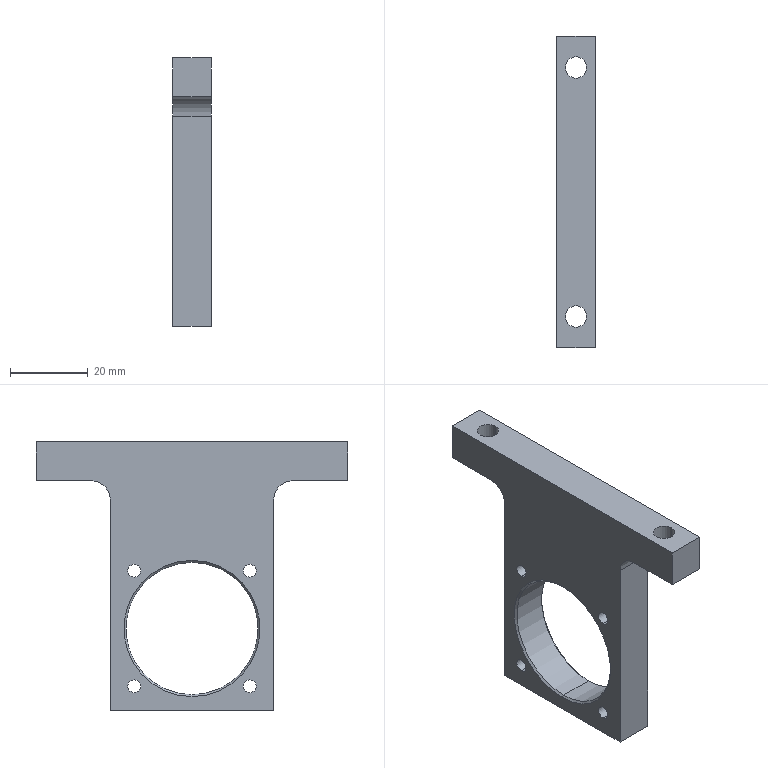Part | SolidWorks | features HoleWzd 2, Chamfer 1, Extrusion 1, Fillet 1, ICE 1 | 1 solid | 30 faces | box 10 x 80 x 69 mm | volume 22964 mm3 | cylinder 16 | plane 10 | cone 4 | commonest cylinder face diameters 3.3 x8 5.5 x4 10 x2 34 x2
STEP:
#1=CARTESIAN_POINT('',(9.5,0.,-31.));
#2=VERTEX_POINT('',#1);
#3=CARTESIAN_POINT('',(9.5,0.,-65.));
#4=VERTEX_POINT('',#3);
#5=CARTESIAN_POINT('',(9.5,0.,-48.));
#6=DIRECTION('',(1.,0.,0.));
#7=DIRECTION('',(0.,0.,1.));
#8=AXIS2_PLACEMENT_3D('',#5,#6,#7);
#9=CIRCLE('',#8,17.);
#10=EDGE_CURVE('',#2,#4,#9,.T.);
#11=ORIENTED_EDGE('',*,*,#10,.F.);
#12=CARTESIAN_POINT('',(10.,0.,-30.5));
#13=VERTEX_POINT('',#12);
#14=CARTESIAN_POINT('',(9.5,0.,-31.));
#15=DIRECTION('',(0.7071,0.,0.7071));
#16=VECTOR('',#15,1000.);
#17=LINE('',#14,#16);
#18=EDGE_CURVE('',#2,#13,#17,.T.);
#19=ORIENTED_EDGE('',*,*,#18,.T.);
#20=CARTESIAN_POINT('',(10.,0.,-65.5));
#21=VERTEX_POINT('',#20);
#22=CARTESIAN_POINT('',(10.,0.,-48.));
#23=DIRECTION('',(-1.,0.,0.));
#24=DIRECTION('',(0.,0.,1.));
#25=AXIS2_PLACEMENT_3D('',#22,#23,#24);
#26=CIRCLE('',#25,17.5);
#27=EDGE_CURVE('',#21,#13,#26,.T.);
#28=ORIENTED_EDGE('',*,*,#27,.F.);
#29=CARTESIAN_POINT('',(9.5,0.,-65.));
#30=DIRECTION('',(0.7071,0.,-0.7071));
#31=VECTOR('',#30,1000.);
#32=LINE('',#29,#31);
#33=EDGE_CURVE('',#4,#21,#32,.T.);
#34=ORIENTED_EDGE('',*,*,#33,.F.);
#35=EDGE_LOOP('',(#11,#19,#28,#34));
#36=FACE_OUTER_BOUND('',#35,.T.);
#37=CARTESIAN_POINT('',(9.5,0.,-48.));
#38=DIRECTION('',(1.,0.,0.));
#39=DIRECTION('',(0.,0.,-1.));
#40=AXIS2_PLACEMENT_3D('',#37,#38,#39);
#41=CONICAL_SURFACE('',#40,17.,0.7854);
#42=ADVANCED_FACE('',(#36),#41,.F.);
#43=CARTESIAN_POINT('',(0.5,0.,-65.));
#44=VERTEX_POINT('',#43);
#45=CARTESIAN_POINT('',(0.5,0.,-31.));
#46=VERTEX_POINT('',#45);
#47=CARTESIAN_POINT('',(0.5,0.,-48.));
#48=DIRECTION('',(-1.,0.,0.));
#49=DIRECTION('',(0.,0.,1.));
#50=AXIS2_PLACEMENT_3D('',#47,#48,#49);
#51=CIRCLE('',#50,17.);
#52=EDGE_CURVE('',#44,#46,#51,.T.);
#53=ORIENTED_EDGE('',*,*,#52,.F.);
#54=CARTESIAN_POINT('',(0.,0.,-65.5));
#55=VERTEX_POINT('',#54);
#56=CARTESIAN_POINT('',(0.,0.,-65.5));
#57=DIRECTION('',(-0.7071,0.,-0.7071));
#58=VECTOR('',#57,1000.);
#59=LINE('',#56,#58);
#60=EDGE_CURVE('',#44,#55,#59,.T.);
#61=ORIENTED_EDGE('',*,*,#60,.T.);
#62=CARTESIAN_POINT('',(0.,0.,-30.5));
#63=VERTEX_POINT('',#62);
#64=CARTESIAN_POINT('',(0.,0.,-48.));
#65=DIRECTION('',(1.,0.,0.));
#66=DIRECTION('',(0.,0.,1.));
#67=AXIS2_PLACEMENT_3D('',#64,#65,#66);
#68=CIRCLE('',#67,17.5);
#69=EDGE_CURVE('',#63,#55,#68,.T.);
#70=ORIENTED_EDGE('',*,*,#69,.F.);
#71=CARTESIAN_POINT('',(0.,0.,-30.5));
#72=DIRECTION('',(-0.7071,0.,0.7071));
#73=VECTOR('',#72,1000.);
#74=LINE('',#71,#73);
#75=EDGE_CURVE('',#46,#63,#74,.T.);
#76=ORIENTED_EDGE('',*,*,#75,.F.);
#77=EDGE_LOOP('',(#53,#61,#70,#76));
#78=FACE_OUTER_BOUND('',#77,.T.);
#79=CARTESIAN_POINT('',(0.,0.,-48.));
#80=DIRECTION('',(-1.,0.,0.));
#81=DIRECTION('',(0.,0.,1.));
#82=AXIS2_PLACEMENT_3D('',#79,#80,#81);
#83=CONICAL_SURFACE('',#82,17.5,0.7854);
#84=ADVANCED_FACE('',(#78),#83,.F.);
#85=CARTESIAN_POINT('',(0.,14.849,-31.501));
#86=VERTEX_POINT('',#85);
#87=CARTESIAN_POINT('',(0.,14.849,-34.801));
#88=VERTEX_POINT('',#87);
#89=CARTESIAN_POINT('',(0.,14.849,-33.151));
#90=DIRECTION('',(1.,0.,0.));
#91=DIRECTION('',(0.,0.,-1.));
#92=AXIS2_PLACEMENT_3D('',#89,#90,#91);
#93=CIRCLE('',#92,1.65);
#94=EDGE_CURVE('',#86,#88,#93,.T.);
#95=ORIENTED_EDGE('',*,*,#94,.F.);
#96=CARTESIAN_POINT('',(10.,14.849,-31.501));
#97=VERTEX_POINT('',#96);
#98=CARTESIAN_POINT('',(10.,14.849,-31.501));
#99=DIRECTION('',(1.,0.,0.));
#100=VECTOR('',#99,1000.);
#101=LINE('',#98,#100);
#102=EDGE_CURVE('',#86,#97,#101,.T.);
#103=ORIENTED_EDGE('',*,*,#102,.T.);
#104=CARTESIAN_POINT('',(10.,14.849,-34.801));
#105=VERTEX_POINT('',#104);
#106=CARTESIAN_POINT('',(10.,14.849,-33.151));
#107=DIRECTION('',(1.,0.,0.));
#108=DIRECTION('',(0.,0.,-1.));
#109=AXIS2_PLACEMENT_3D('',#106,#107,#108);
#110=CIRCLE('',#109,1.65);
#111=EDGE_CURVE('',#97,#105,#110,.T.);
#112=ORIENTED_EDGE('',*,*,#111,.T.);
#113=CARTESIAN_POINT('',(10.,14.849,-34.801));
#114=DIRECTION('',(1.,0.,0.));
#115=VECTOR('',#114,1000.);
#116=LINE('',#113,#115);
#117=EDGE_CURVE('',#88,#105,#116,.T.);
#118=ORIENTED_EDGE('',*,*,#117,.F.);
#119=EDGE_LOOP('',(#95,#103,#112,#118));
#120=FACE_OUTER_BOUND('',#119,.T.);
#121=CARTESIAN_POINT('',(10.,14.849,-33.151));
#122=DIRECTION('',(1.,0.,0.));
#123=DIRECTION('',(0.,0.,-1.));
#124=AXIS2_PLACEMENT_3D('',#121,#122,#123);
#125=CYLINDRICAL_SURFACE('',#124,1.65);
#126=ADVANCED_FACE('',(#120),#125,.F.);
#127=CARTESIAN_POINT('',(0.,14.849,-61.199));
#128=VERTEX_POINT('',#127);
#129=CARTESIAN_POINT('',(0.,14.849,-64.499));
#130=VERTEX_POINT('',#129);
#131=CARTESIAN_POINT('',(0.,14.849,-62.849));
#132=DIRECTION('',(1.,0.,0.));
#133=DIRECTION('',(0.,0.,-1.));
#134=AXIS2_PLACEMENT_3D('',#131,#132,#133);
#135=CIRCLE('',#134,1.65);
#136=EDGE_CURVE('',#128,#130,#135,.T.);
#137=ORIENTED_EDGE('',*,*,#136,.F.);
#138=CARTESIAN_POINT('',(10.,14.849,-61.199));
#139=VERTEX_POINT('',#138);
#140=CARTESIAN_POINT('',(10.,14.849,-61.199));
#141=DIRECTION('',(1.,0.,0.));
#142=VECTOR('',#141,1000.);
#143=LINE('',#140,#142);
#144=EDGE_CURVE('',#128,#139,#143,.T.);
#145=ORIENTED_EDGE('',*,*,#144,.T.);
#146=CARTESIAN_POINT('',(10.,14.849,-64.499));
#147=VERTEX_POINT('',#146);
#148=CARTESIAN_POINT('',(10.,14.849,-62.849));
#149=DIRECTION('',(1.,0.,0.));
#150=DIRECTION('',(0.,0.,-1.));
#151=AXIS2_PLACEMENT_3D('',#148,#149,#150);
#152=CIRCLE('',#151,1.65);
#153=EDGE_CURVE('',#139,#147,#152,.T.);
#154=ORIENTED_EDGE('',*,*,#153,.T.);
#155=CARTESIAN_POINT('',(10.,14.849,-64.499));
#156=DIRECTION('',(1.,0.,0.));
#157=VECTOR('',#156,1000.);
#158=LINE('',#155,#157);
#159=EDGE_CURVE('',#130,#147,#158,.T.);
#160=ORIENTED_EDGE('',*,*,#159,.F.);
#161=EDGE_LOOP('',(#137,#145,#154,#160));
#162=FACE_OUTER_BOUND('',#161,.T.);
#163=CARTESIAN_POINT('',(10.,14.849,-62.849));
#164=DIRECTION('',(1.,0.,0.));
#165=DIRECTION('',(0.,0.,-1.));
#166=AXIS2_PLACEMENT_3D('',#163,#164,#165);
#167=CYLINDRICAL_SURFACE('',#166,1.65);
#168=ADVANCED_FACE('',(#162),#167,.F.);
#169=CARTESIAN_POINT('',(0.,-14.849,-61.199));
#170=VERTEX_POINT('',#169);
#171=CARTESIAN_POINT('',(0.,-14.849,-64.499));
#172=VERTEX_POINT('',#171);
#173=CARTESIAN_POINT('',(0.,-14.849,-62.849));
#174=DIRECTION('',(1.,0.,0.));
#175=DIRECTION('',(0.,0.,-1.));
#176=AXIS2_PLACEMENT_3D('',#173,#174,#175);
#177=CIRCLE('',#176,1.65);
#178=EDGE_CURVE('',#170,#172,#177,.T.);
#179=ORIENTED_EDGE('',*,*,#178,.F.);
#180=CARTESIAN_POINT('',(10.,-14.849,-61.199));
#181=VERTEX_POINT('',#180);
#182=CARTESIAN_POINT('',(10.,-14.849,-61.199));
#183=DIRECTION('',(1.,0.,0.));
#184=VECTOR('',#183,1000.);
#185=LINE('',#182,#184);
#186=EDGE_CURVE('',#170,#181,#185,.T.);
#187=ORIENTED_EDGE('',*,*,#186,.T.);
#188=CARTESIAN_POINT('',(10.,-14.849,-64.499));
#189=VERTEX_POINT('',#188);
#190=CARTESIAN_POINT('',(10.,-14.849,-62.849));
#191=DIRECTION('',(1.,0.,0.));
#192=DIRECTION('',(0.,0.,-1.));
#193=AXIS2_PLACEMENT_3D('',#190,#191,#192);
#194=CIRCLE('',#193,1.65);
#195=EDGE_CURVE('',#181,#189,#194,.T.);
#196=ORIENTED_EDGE('',*,*,#195,.T.);
#197=CARTESIAN_POINT('',(10.,-14.849,-64.499));
#198=DIRECTION('',(1.,0.,0.));
#199=VECTOR('',#198,1000.);
#200=LINE('',#197,#199);
#201=EDGE_CURVE('',#172,#189,#200,.T.);
#202=ORIENTED_EDGE('',*,*,#201,.F.);
#203=EDGE_LOOP('',(#179,#187,#196,#202));
#204=FACE_OUTER_BOUND('',#203,.T.);
#205=CARTESIAN_POINT('',(10.,-14.849,-62.849));
#206=DIRECTION('',(1.,0.,0.));
#207=DIRECTION('',(0.,0.,-1.));
#208=AXIS2_PLACEMENT_3D('',#205,#206,#207);
#209=CYLINDRICAL_SURFACE('',#208,1.65);
#210=ADVANCED_FACE('',(#204),#209,.F.);
#211=CARTESIAN_POINT('',(0.,-14.849,-31.501));
#212=VERTEX_POINT('',#211);
#213=CARTESIAN_POINT('',(0.,-14.849,-34.801));
#214=VERTEX_POINT('',#213);
#215=CARTESIAN_POINT('',(0.,-14.849,-33.151));
#216=DIRECTION('',(1.,0.,0.));
#217=DIRECTION('',(0.,0.,-1.));
#218=AXIS2_PLACEMENT_3D('',#215,#216,#217);
#219=CIRCLE('',#218,1.65);
#220=EDGE_CURVE('',#212,#214,#219,.T.);
#221=ORIENTED_EDGE('',*,*,#220,.F.);
#222=CARTESIAN_POINT('',(10.,-14.849,-31.501));
#223=VERTEX_POINT('',#222);
#224=CARTESIAN_POINT('',(10.,-14.849,-31.501));
#225=DIRECTION('',(1.,0.,0.));
#226=VECTOR('',#225,1000.);
#227=LINE('',#224,#226);
#228=EDGE_CURVE('',#212,#223,#227,.T.);
#229=ORIENTED_EDGE('',*,*,#228,.T.);
#230=CARTESIAN_POINT('',(10.,-14.849,-34.801));
#231=VERTEX_POINT('',#230);
#232=CARTESIAN_POINT('',(10.,-14.849,-33.151));
#233=DIRECTION('',(1.,0.,0.));
#234=DIRECTION('',(0.,0.,-1.));
#235=AXIS2_PLACEMENT_3D('',#232,#233,#234);
#236=CIRCLE('',#235,1.65);
#237=EDGE_CURVE('',#223,#231,#236,.T.);
#238=ORIENTED_EDGE('',*,*,#237,.T.);
#239=CARTESIAN_POINT('',(10.,-14.849,-34.801));
#240=DIRECTION('',(1.,0.,0.));
#241=VECTOR('',#240,1000.);
#242=LINE('',#239,#241);
#243=EDGE_CURVE('',#214,#231,#242,.T.);
#244=ORIENTED_EDGE('',*,*,#243,.F.);
#245=EDGE_LOOP('',(#221,#229,#238,#244));
#246=FACE_OUTER_BOUND('',#245,.T.);
#247=CARTESIAN_POINT('',(10.,-14.849,-33.151));
#248=DIRECTION('',(1.,0.,0.));
#249=DIRECTION('',(0.,0.,-1.));
#250=AXIS2_PLACEMENT_3D('',#247,#248,#249);
#251=CYLINDRICAL_SURFACE('',#250,1.65);
#252=ADVANCED_FACE('',(#246),#251,.F.);
#253=CARTESIAN_POINT('',(2.25,32.,-10.));
#254=VERTEX_POINT('',#253);
#255=CARTESIAN_POINT('',(7.75,32.,-10.));
#256=VERTEX_POINT('',#255);
#257=CARTESIAN_POINT('',(5.,32.,-10.));
#258=DIRECTION('',(0.,0.,1.));
#259=DIRECTION('',(0.,-1.,0.));
#260=AXIS2_PLACEMENT_3D('',#257,#258,#259);
#261=CIRCLE('',#260,2.75);
#262=EDGE_CURVE('',#254,#256,#261,.T.);
#263=ORIENTED_EDGE('',*,*,#262,.F.);
#264=CARTESIAN_POINT('',(2.25,32.,0.));
#265=VERTEX_POINT('',#264);
#266=CARTESIAN_POINT('',(2.25,32.,0.));
#267=DIRECTION('',(0.,0.,1.));
#268=VECTOR('',#267,1000.);
#269=LINE('',#266,#268);
#270=EDGE_CURVE('',#254,#265,#269,.T.);
#271=ORIENTED_EDGE('',*,*,#270,.T.);
#272=CARTESIAN_POINT('',(7.75,32.,0.));
#273=VERTEX_POINT('',#272);
#274=CARTESIAN_POINT('',(5.,32.,0.));
#275=DIRECTION('',(0.,0.,1.));
#276=DIRECTION('',(1.,0.,0.));
#277=AXIS2_PLACEMENT_3D('',#274,#275,#276);
#278=CIRCLE('',#277,2.75);
#279=EDGE_CURVE('',#265,#273,#278,.T.);
#280=ORIENTED_EDGE('',*,*,#279,.T.);
#281=CARTESIAN_POINT('',(7.75,32.,0.));
#282=DIRECTION('',(0.,0.,1.));
#283=VECTOR('',#282,1000.);
#284=LINE('',#281,#283);
#285=EDGE_CURVE('',#256,#273,#284,.T.);
#286=ORIENTED_EDGE('',*,*,#285,.F.);
#287=EDGE_LOOP('',(#263,#271,#280,#286));
#288=FACE_OUTER_BOUND('',#287,.T.);
#289=CARTESIAN_POINT('',(5.,32.,0.));
#290=DIRECTION('',(0.,0.,1.));
#291=DIRECTION('',(1.,0.,0.));
#292=AXIS2_PLACEMENT_3D('',#289,#290,#291);
#293=CYLINDRICAL_SURFACE('',#292,2.75);
#294=ADVANCED_FACE('',(#288),#293,.F.);
#295=CARTESIAN_POINT('',(2.25,-32.,-10.));
#296=VERTEX_POINT('',#295);
#297=CARTESIAN_POINT('',(7.75,-32.,-10.));
#298=VERTEX_POINT('',#297);
#299=CARTESIAN_POINT('',(5.,-32.,-10.));
#300=DIRECTION('',(0.,0.,1.));
#301=DIRECTION('',(0.,-1.,0.));
#302=AXIS2_PLACEMENT_3D('',#299,#300,#301);
#303=CIRCLE('',#302,2.75);
#304=EDGE_CURVE('',#296,#298,#303,.T.);
#305=ORIENTED_EDGE('',*,*,#304,.F.);
#306=CARTESIAN_POINT('',(2.25,-32.,0.));
#307=VERTEX_POINT('',#306);
#308=CARTESIAN_POINT('',(2.25,-32.,0.));
#309=DIRECTION('',(0.,0.,1.));
#310=VECTOR('',#309,1000.);
#311=LINE('',#308,#310);
#312=EDGE_CURVE('',#296,#307,#311,.T.);
#313=ORIENTED_EDGE('',*,*,#312,.T.);
#314=CARTESIAN_POINT('',(7.75,-32.,0.));
#315=VERTEX_POINT('',#314);
#316=CARTESIAN_POINT('',(5.,-32.,0.));
#317=DIRECTION('',(0.,0.,1.));
#318=DIRECTION('',(1.,0.,0.));
#319=AXIS2_PLACEMENT_3D('',#316,#317,#318);
#320=CIRCLE('',#319,2.75);
#321=EDGE_CURVE('',#307,#315,#320,.T.);
#322=ORIENTED_EDGE('',*,*,#321,.T.);
#323=CARTESIAN_POINT('',(7.75,-32.,0.));
#324=DIRECTION('',(0.,0.,1.));
#325=VECTOR('',#324,1000.);
#326=LINE('',#323,#325);
#327=EDGE_CURVE('',#298,#315,#326,.T.);
#328=ORIENTED_EDGE('',*,*,#327,.F.);
#329=EDGE_LOOP('',(#305,#313,#322,#328));
#330=FACE_OUTER_BOUND('',#329,.T.);
#331=CARTESIAN_POINT('',(5.,-32.,0.));
#332=DIRECTION('',(0.,0.,1.));
#333=DIRECTION('',(1.,0.,0.));
#334=AXIS2_PLACEMENT_3D('',#331,#332,#333);
#335=CYLINDRICAL_SURFACE('',#334,2.75);
#336=ADVANCED_FACE('',(#330),#335,.F.);
#337=ORIENTED_EDGE('',*,*,#52,.T.);
#338=CARTESIAN_POINT('',(0.,0.,-31.));
#339=DIRECTION('',(1.,0.,0.));
#340=VECTOR('',#339,1000.);
#341=LINE('',#338,#340);
#342=EDGE_CURVE('',#46,#2,#341,.T.);
#343=ORIENTED_EDGE('',*,*,#342,.T.);
#344=ORIENTED_EDGE('',*,*,#10,.T.);
#345=CARTESIAN_POINT('',(0.,0.,-65.));
#346=DIRECTION('',(1.,0.,0.));
#347=VECTOR('',#346,1000.);
#348=LINE('',#345,#347);
#349=EDGE_CURVE('',#44,#4,#348,.T.);
#350=ORIENTED_EDGE('',*,*,#349,.F.);
#351=EDGE_LOOP('',(#337,#343,#344,#350));
#352=FACE_OUTER_BOUND('',#351,.T.);
#353=CARTESIAN_POINT('',(0.,0.,-48.));
#354=DIRECTION('',(1.,0.,0.));
#355=DIRECTION('',(0.,0.,-1.));
#356=AXIS2_PLACEMENT_3D('',#353,#354,#355);
#357=CYLINDRICAL_SURFACE('',#356,17.);
#358=ADVANCED_FACE('',(#352),#357,.F.);
#359=CARTESIAN_POINT('',(0.,-40.,0.));
#360=VERTEX_POINT('',#359);
#361=CARTESIAN_POINT('',(0.,-40.,-10.));
#362=VERTEX_POINT('',#361);
#363=CARTESIAN_POINT('',(0.,-40.,-10.));
#364=DIRECTION('',(0.,0.,-1.));
#365=VECTOR('',#364,1000.);
#366=LINE('',#363,#365);
#367=EDGE_CURVE('',#360,#362,#366,.T.);
#368=ORIENTED_EDGE('',*,*,#367,.T.);
#369=CARTESIAN_POINT('',(10.,-40.,-10.));
#370=VERTEX_POINT('',#369);
#371=CARTESIAN_POINT('',(10.,-40.,-10.));
#372=DIRECTION('',(-1.,0.,0.));
#373=VECTOR('',#372,1000.);
#374=LINE('',#371,#373);
#375=EDGE_CURVE('',#370,#362,#374,.T.);
#376=ORIENTED_EDGE('',*,*,#375,.F.);
#377=CARTESIAN_POINT('',(10.,-40.,0.));
#378=VERTEX_POINT('',#377);
#379=CARTESIAN_POINT('',(10.,-40.,-10.));
#380=DIRECTION('',(0.,0.,-1.));
#381=VECTOR('',#380,1000.);
#382=LINE('',#379,#381);
#383=EDGE_CURVE('',#378,#370,#382,.T.);
#384=ORIENTED_EDGE('',*,*,#383,.F.);
#385=CARTESIAN_POINT('',(10.,-40.,0.));
#386=DIRECTION('',(-1.,0.,0.));
#387=VECTOR('',#386,1000.);
#388=LINE('',#385,#387);
#389=EDGE_CURVE('',#378,#360,#388,.T.);
#390=ORIENTED_EDGE('',*,*,#389,.T.);
#391=EDGE_LOOP('',(#368,#376,#384,#390));
#392=FACE_OUTER_BOUND('',#391,.T.);
#393=CARTESIAN_POINT('',(10.,-40.,-10.));
#394=DIRECTION('',(0.,1.,0.));
#395=DIRECTION('',(0.,0.,1.));
#396=AXIS2_PLACEMENT_3D('',#393,#394,#395);
#397=PLANE('',#396);
#398=ADVANCED_FACE('',(#392),#397,.F.);
#399=CARTESIAN_POINT('',(5.,-32.,-10.));
#400=DIRECTION('',(0.,0.,1.));
#401=DIRECTION('',(0.,-1.,0.));
#402=AXIS2_PLACEMENT_3D('',#399,#400,#401);
#403=CIRCLE('',#402,2.75);
#404=EDGE_CURVE('',#298,#296,#403,.T.);
#405=ORIENTED_EDGE('',*,*,#404,.T.);
#406=ORIENTED_EDGE('',*,*,#304,.T.);
#407=EDGE_LOOP('',(#405,#406));
#408=FACE_BOUND('',#407,.T.);
#409=CARTESIAN_POINT('',(0.,-26.,-10.));
#410=VERTEX_POINT('',#409);
#411=CARTESIAN_POINT('',(0.,-21.,-10.));
#412=DIRECTION('',(0.,1.,0.));
#413=VECTOR('',#412,1000.);
#414=LINE('',#411,#413);
#415=EDGE_CURVE('',#362,#410,#414,.T.);
#416=ORIENTED_EDGE('',*,*,#415,.T.);
#417=CARTESIAN_POINT('',(10.,-26.,-10.));
#418=VERTEX_POINT('',#417);
#419=CARTESIAN_POINT('',(10.,-26.,-10.));
#420=DIRECTION('',(1.,0.,0.));
#421=VECTOR('',#420,1000.);
#422=LINE('',#419,#421);
#423=EDGE_CURVE('',#410,#418,#422,.T.);
#424=ORIENTED_EDGE('',*,*,#423,.T.);
#425=CARTESIAN_POINT('',(10.,-21.,-10.));
#426=DIRECTION('',(0.,1.,0.));
#427=VECTOR('',#426,1000.);
#428=LINE('',#425,#427);
#429=EDGE_CURVE('',#370,#418,#428,.T.);
#430=ORIENTED_EDGE('',*,*,#429,.F.);
#431=ORIENTED_EDGE('',*,*,#375,.T.);
#432=EDGE_LOOP('',(#416,#424,#430,#431));
#433=FACE_OUTER_BOUND('',#432,.T.);
#434=CARTESIAN_POINT('',(10.,-21.,-10.));
#435=DIRECTION('',(0.,0.,1.));
#436=DIRECTION('',(0.,-1.,0.));
#437=AXIS2_PLACEMENT_3D('',#434,#435,#436);
#438=PLANE('',#437);
#439=ADVANCED_FACE('',(#408,#433),#438,.F.);
#440=CARTESIAN_POINT('',(10.,-21.,-15.));
#441=VERTEX_POINT('',#440);
#442=CARTESIAN_POINT('',(10.,-21.,-69.));
#443=VERTEX_POINT('',#442);
#444=CARTESIAN_POINT('',(10.,-21.,-69.));
#445=DIRECTION('',(0.,0.,-1.));
#446=VECTOR('',#445,1000.);
#447=LINE('',#444,#446);
#448=EDGE_CURVE('',#441,#443,#447,.T.);
#449=ORIENTED_EDGE('',*,*,#448,.F.);
#450=CARTESIAN_POINT('',(0.,-21.,-15.));
#451=VERTEX_POINT('',#450);
#452=CARTESIAN_POINT('',(0.,-21.,-15.));
#453=DIRECTION('',(-1.,0.,0.));
#454=VECTOR('',#453,1000.);
#455=LINE('',#452,#454);
#456=EDGE_CURVE('',#441,#451,#455,.T.);
#457=ORIENTED_EDGE('',*,*,#456,.T.);
#458=CARTESIAN_POINT('',(0.,-21.,-69.));
#459=VERTEX_POINT('',#458);
#460=CARTESIAN_POINT('',(0.,-21.,-69.));
#461=DIRECTION('',(0.,0.,-1.));
#462=VECTOR('',#461,1000.);
#463=LINE('',#460,#462);
#464=EDGE_CURVE('',#451,#459,#463,.T.);
#465=ORIENTED_EDGE('',*,*,#464,.T.);
#466=CARTESIAN_POINT('',(10.,-21.,-69.));
#467=DIRECTION('',(-1.,0.,0.));
#468=VECTOR('',#467,1000.);
#469=LINE('',#466,#468);
#470=EDGE_CURVE('',#443,#459,#469,.T.);
#471=ORIENTED_EDGE('',*,*,#470,.F.);
#472=EDGE_LOOP('',(#449,#457,#465,#471));
#473=FACE_OUTER_BOUND('',#472,.T.);
#474=CARTESIAN_POINT('',(10.,-21.,-69.));
#475=DIRECTION('',(0.,1.,0.));
#476=DIRECTION('',(0.,0.,1.));
#477=AXIS2_PLACEMENT_3D('',#474,#475,#476);
#478=PLANE('',#477);
#479=ADVANCED_FACE('',(#473),#478,.F.);
#480=CARTESIAN_POINT('',(0.,21.,-69.));
#481=VERTEX_POINT('',#480);
#482=CARTESIAN_POINT('',(0.,21.,-69.));
#483=DIRECTION('',(0.,1.,0.));
#484=VECTOR('',#483,1000.);
#485=LINE('',#482,#484);
#486=EDGE_CURVE('',#459,#481,#485,.T.);
#487=ORIENTED_EDGE('',*,*,#486,.T.);
#488=CARTESIAN_POINT('',(10.,21.,-69.));
#489=VERTEX_POINT('',#488);
#490=CARTESIAN_POINT('',(10.,21.,-69.));
#491=DIRECTION('',(-1.,0.,0.));
#492=VECTOR('',#491,1000.);
#493=LINE('',#490,#492);
#494=EDGE_CURVE('',#489,#481,#493,.T.);
#495=ORIENTED_EDGE('',*,*,#494,.F.);
#496=CARTESIAN_POINT('',(10.,21.,-69.));
#497=DIRECTION('',(0.,1.,0.));
#498=VECTOR('',#497,1000.);
#499=LINE('',#496,#498);
#500=EDGE_CURVE('',#443,#489,#499,.T.);
#501=ORIENTED_EDGE('',*,*,#500,.F.);
#502=ORIENTED_EDGE('',*,*,#470,.T.);
#503=EDGE_LOOP('',(#487,#495,#501,#502));
#504=FACE_OUTER_BOUND('',#503,.T.);
#505=CARTESIAN_POINT('',(10.,21.,-69.));
#506=DIRECTION('',(0.,0.,1.));
#507=DIRECTION('',(1.,0.,0.));
#508=AXIS2_PLACEMENT_3D('',#505,#506,#507);
#509=PLANE('',#508);
#510=ADVANCED_FACE('',(#504),#509,.F.);
#511=CARTESIAN_POINT('',(0.,21.,-15.));
#512=VERTEX_POINT('',#511);
#513=CARTESIAN_POINT('',(0.,21.,-10.));
#514=DIRECTION('',(0.,0.,1.));
#515=VECTOR('',#514,1000.);
#516=LINE('',#513,#515);
#517=EDGE_CURVE('',#481,#512,#516,.T.);
#518=ORIENTED_EDGE('',*,*,#517,.T.);
#519=CARTESIAN_POINT('',(10.,21.,-15.));
#520=VERTEX_POINT('',#519);
#521=CARTESIAN_POINT('',(10.,21.,-15.));
#522=DIRECTION('',(1.,0.,0.));
#523=VECTOR('',#522,1000.);
#524=LINE('',#521,#523);
#525=EDGE_CURVE('',#512,#520,#524,.T.);
#526=ORIENTED_EDGE('',*,*,#525,.T.);
#527=CARTESIAN_POINT('',(10.,21.,-10.));
#528=DIRECTION('',(0.,0.,1.));
#529=VECTOR('',#528,1000.);
#530=LINE('',#527,#529);
#531=EDGE_CURVE('',#489,#520,#530,.T.);
#532=ORIENTED_EDGE('',*,*,#531,.F.);
#533=ORIENTED_EDGE('',*,*,#494,.T.);
#534=EDGE_LOOP('',(#518,#526,#532,#533));
#535=FACE_OUTER_BOUND('',#534,.T.);
#536=CARTESIAN_POINT('',(10.,21.,-10.));
#537=DIRECTION('',(0.,-1.,0.));
#538=DIRECTION('',(0.,0.,-1.));
#539=AXIS2_PLACEMENT_3D('',#536,#537,#538);
#540=PLANE('',#539);
#541=ADVANCED_FACE('',(#535),#540,.F.);
#542=CARTESIAN_POINT('',(5.,32.,-10.));
#543=DIRECTION('',(0.,0.,1.));
#544=DIRECTION('',(0.,-1.,0.));
#545=AXIS2_PLACEMENT_3D('',#542,#543,#544);
#546=CIRCLE('',#545,2.75);
#547=EDGE_CURVE('',#256,#254,#546,.T.);
#548=ORIENTED_EDGE('',*,*,#547,.T.);
#549=ORIENTED_EDGE('',*,*,#262,.T.);
#550=EDGE_LOOP('',(#548,#549));
#551=FACE_BOUND('',#550,.T.);
#552=CARTESIAN_POINT('',(10.,26.,-10.));
#553=VERTEX_POINT('',#552);
#554=CARTESIAN_POINT('',(10.,40.,-10.));
#555=VERTEX_POINT('',#554);
#556=CARTESIAN_POINT('',(10.,40.,-10.));
#557=DIRECTION('',(0.,1.,0.));
#558=VECTOR('',#557,1000.);
#559=LINE('',#556,#558);
#560=EDGE_CURVE('',#553,#555,#559,.T.);
#561=ORIENTED_EDGE('',*,*,#560,.F.);
#562=CARTESIAN_POINT('',(0.,26.,-10.));
#563=VERTEX_POINT('',#562);
#564=CARTESIAN_POINT('',(0.,26.,-10.));
#565=DIRECTION('',(-1.,0.,0.));
#566=VECTOR('',#565,1000.);
#567=LINE('',#564,#566);
#568=EDGE_CURVE('',#553,#563,#567,.T.);
#569=ORIENTED_EDGE('',*,*,#568,.T.);
#570=CARTESIAN_POINT('',(0.,40.,-10.));
#571=VERTEX_POINT('',#570);
#572=CARTESIAN_POINT('',(0.,40.,-10.));
#573=DIRECTION('',(0.,1.,0.));
#574=VECTOR('',#573,1000.);
#575=LINE('',#572,#574);
#576=EDGE_CURVE('',#563,#571,#575,.T.);
#577=ORIENTED_EDGE('',*,*,#576,.T.);
#578=CARTESIAN_POINT('',(10.,40.,-10.));
#579=DIRECTION('',(-1.,0.,0.));
#580=VECTOR('',#579,1000.);
#581=LINE('',#578,#580);
#582=EDGE_CURVE('',#555,#571,#581,.T.);
#583=ORIENTED_EDGE('',*,*,#582,.F.);
#584=EDGE_LOOP('',(#561,#569,#577,#583));
#585=FACE_OUTER_BOUND('',#584,.T.);
#586=CARTESIAN_POINT('',(10.,40.,-10.));
#587=DIRECTION('',(0.,0.,1.));
#588=DIRECTION('',(0.,-1.,0.));
#589=AXIS2_PLACEMENT_3D('',#586,#587,#588);
#590=PLANE('',#589);
#591=ADVANCED_FACE('',(#551,#585),#590,.F.);
#592=CARTESIAN_POINT('',(0.,40.,0.));
#593=VERTEX_POINT('',#592);
#594=CARTESIAN_POINT('',(0.,40.,0.));
#595=DIRECTION('',(0.,0.,1.));
#596=VECTOR('',#595,1000.);
#597=LINE('',#594,#596);
#598=EDGE_CURVE('',#571,#593,#597,.T.);
#599=ORIENTED_EDGE('',*,*,#598,.T.);
#600=CARTESIAN_POINT('',(10.,40.,0.));
#601=VERTEX_POINT('',#600);
#602=CARTESIAN_POINT('',(10.,40.,0.));
#603=DIRECTION('',(-1.,0.,0.));
#604=VECTOR('',#603,1000.);
#605=LINE('',#602,#604);
#606=EDGE_CURVE('',#601,#593,#605,.T.);
#607=ORIENTED_EDGE('',*,*,#606,.F.);
#608=CARTESIAN_POINT('',(10.,40.,0.));
#609=DIRECTION('',(0.,0.,1.));
#610=VECTOR('',#609,1000.);
#611=LINE('',#608,#610);
#612=EDGE_CURVE('',#555,#601,#611,.T.);
#613=ORIENTED_EDGE('',*,*,#612,.F.);
#614=ORIENTED_EDGE('',*,*,#582,.T.);
#615=EDGE_LOOP('',(#599,#607,#613,#614));
#616=FACE_OUTER_BOUND('',#615,.T.);
#617=CARTESIAN_POINT('',(10.,40.,0.));
#618=DIRECTION('',(0.,-1.,0.));
#619=DIRECTION('',(0.,0.,-1.));
#620=AXIS2_PLACEMENT_3D('',#617,#618,#619);
#621=PLANE('',#620);
#622=ADVANCED_FACE('',(#616),#621,.F.);
#623=CARTESIAN_POINT('',(5.,32.,0.));
#624=DIRECTION('',(0.,0.,1.));
#625=DIRECTION('',(1.,0.,0.));
#626=AXIS2_PLACEMENT_3D('',#623,#624,#625);
#627=CIRCLE('',#626,2.75);
#628=EDGE_CURVE('',#273,#265,#627,.T.);
#629=ORIENTED_EDGE('',*,*,#628,.F.);
#630=ORIENTED_EDGE('',*,*,#279,.F.);
#631=EDGE_LOOP('',(#629,#630));
#632=FACE_BOUND('',#631,.T.);
#633=CARTESIAN_POINT('',(5.,-32.,0.));
#634=DIRECTION('',(0.,0.,1.));
#635=DIRECTION('',(1.,0.,0.));
#636=AXIS2_PLACEMENT_3D('',#633,#634,#635);
#637=CIRCLE('',#636,2.75);
#638=EDGE_CURVE('',#315,#307,#637,.T.);
#639=ORIENTED_EDGE('',*,*,#638,.F.);
#640=ORIENTED_EDGE('',*,*,#321,.F.);
#641=EDGE_LOOP('',(#639,#640));
#642=FACE_BOUND('',#641,.T.);
#643=CARTESIAN_POINT('',(0.,-40.,0.));
#644=DIRECTION('',(0.,-1.,0.));
#645=VECTOR('',#644,1000.);
#646=LINE('',#643,#645);
#647=EDGE_CURVE('',#593,#360,#646,.T.);
#648=ORIENTED_EDGE('',*,*,#647,.T.);
#649=ORIENTED_EDGE('',*,*,#389,.F.);
#650=CARTESIAN_POINT('',(10.,-40.,0.));
#651=DIRECTION('',(0.,-1.,0.));
#652=VECTOR('',#651,1000.);
#653=LINE('',#650,#652);
#654=EDGE_CURVE('',#601,#378,#653,.T.);
#655=ORIENTED_EDGE('',*,*,#654,.F.);
#656=ORIENTED_EDGE('',*,*,#606,.T.);
#657=EDGE_LOOP('',(#648,#649,#655,#656));
#658=FACE_OUTER_BOUND('',#657,.T.);
#659=CARTESIAN_POINT('',(10.,-40.,0.));
#660=DIRECTION('',(0.,0.,-1.));
#661=DIRECTION('',(-1.,0.,0.));
#662=AXIS2_PLACEMENT_3D('',#659,#660,#661);
#663=PLANE('',#662);
#664=ADVANCED_FACE('',(#632,#642,#658),#663,.F.);
#665=ORIENTED_EDGE('',*,*,#27,.T.);
#666=CARTESIAN_POINT('',(10.,0.,-48.));
#667=DIRECTION('',(-1.,0.,0.));
#668=DIRECTION('',(0.,0.,1.));
#669=AXIS2_PLACEMENT_3D('',#666,#667,#668);
#670=CIRCLE('',#669,17.5);
#671=EDGE_CURVE('',#13,#21,#670,.T.);
#672=ORIENTED_EDGE('',*,*,#671,.T.);
#673=EDGE_LOOP('',(#665,#672));
#674=FACE_BOUND('',#673,.T.);
#675=CARTESIAN_POINT('',(10.,14.849,-33.151));
#676=DIRECTION('',(1.,0.,0.));
#677=DIRECTION('',(0.,0.,-1.));
#678=AXIS2_PLACEMENT_3D('',#675,#676,#677);
#679=CIRCLE('',#678,1.65);
#680=EDGE_CURVE('',#105,#97,#679,.T.);
#681=ORIENTED_EDGE('',*,*,#680,.F.);
#682=ORIENTED_EDGE('',*,*,#111,.F.);
#683=EDGE_LOOP('',(#681,#682));
#684=FACE_BOUND('',#683,.T.);
#685=CARTESIAN_POINT('',(10.,14.849,-62.849));
#686=DIRECTION('',(1.,0.,0.));
#687=DIRECTION('',(0.,0.,-1.));
#688=AXIS2_PLACEMENT_3D('',#685,#686,#687);
#689=CIRCLE('',#688,1.65);
#690=EDGE_CURVE('',#147,#139,#689,.T.);
#691=ORIENTED_EDGE('',*,*,#690,.F.);
#692=ORIENTED_EDGE('',*,*,#153,.F.);
#693=EDGE_LOOP('',(#691,#692));
#694=FACE_BOUND('',#693,.T.);
#695=CARTESIAN_POINT('',(10.,-14.849,-62.849));
#696=DIRECTION('',(1.,0.,0.));
#697=DIRECTION('',(0.,0.,-1.));
#698=AXIS2_PLACEMENT_3D('',#695,#696,#697);
#699=CIRCLE('',#698,1.65);
#700=EDGE_CURVE('',#189,#181,#699,.T.);
#701=ORIENTED_EDGE('',*,*,#700,.F.);
#702=ORIENTED_EDGE('',*,*,#195,.F.);
#703=EDGE_LOOP('',(#701,#702));
#704=FACE_BOUND('',#703,.T.);
#705=CARTESIAN_POINT('',(10.,-14.849,-33.151));
#706=DIRECTION('',(1.,0.,0.));
#707=DIRECTION('',(0.,0.,-1.));
#708=AXIS2_PLACEMENT_3D('',#705,#706,#707);
#709=CIRCLE('',#708,1.65);
#710=EDGE_CURVE('',#231,#223,#709,.T.);
#711=ORIENTED_EDGE('',*,*,#710,.F.);
#712=ORIENTED_EDGE('',*,*,#237,.F.);
#713=EDGE_LOOP('',(#711,#712));
#714=FACE_BOUND('',#713,.T.);
#715=ORIENTED_EDGE('',*,*,#383,.T.);
#716=ORIENTED_EDGE('',*,*,#429,.T.);
#717=CARTESIAN_POINT('',(10.,-26.,-15.));
#718=DIRECTION('',(-1.,0.,0.));
#719=DIRECTION('',(0.,0.,1.));
#720=AXIS2_PLACEMENT_3D('',#717,#718,#719);
#721=CIRCLE('',#720,5.);
#722=EDGE_CURVE('',#418,#441,#721,.T.);
#723=ORIENTED_EDGE('',*,*,#722,.T.);
#724=ORIENTED_EDGE('',*,*,#448,.T.);
#725=ORIENTED_EDGE('',*,*,#500,.T.);
#726=ORIENTED_EDGE('',*,*,#531,.T.);
#727=CARTESIAN_POINT('',(10.,26.,-15.));
#728=DIRECTION('',(-1.,0.,0.));
#729=DIRECTION('',(0.,0.,1.));
#730=AXIS2_PLACEMENT_3D('',#727,#728,#729);
#731=CIRCLE('',#730,5.);
#732=EDGE_CURVE('',#520,#553,#731,.T.);
#733=ORIENTED_EDGE('',*,*,#732,.T.);
#734=ORIENTED_EDGE('',*,*,#560,.T.);
#735=ORIENTED_EDGE('',*,*,#612,.T.);
#736=ORIENTED_EDGE('',*,*,#654,.T.);
#737=EDGE_LOOP('',(#715,#716,#723,#724,#725,#726,#733,#734,#735,#736));
#738=FACE_OUTER_BOUND('',#737,.T.);
#739=CARTESIAN_POINT('',(10.,-40.,0.));
#740=DIRECTION('',(-1.,0.,0.));
#741=DIRECTION('',(0.,0.,1.));
#742=AXIS2_PLACEMENT_3D('',#739,#740,#741);
#743=PLANE('',#742);
#744=ADVANCED_FACE('',(#674,#684,#694,#704,#714,#738),#743,.F.);
#745=ORIENTED_EDGE('',*,*,#69,.T.);
#746=CARTESIAN_POINT('',(0.,0.,-48.));
#747=DIRECTION('',(1.,0.,0.));
#748=DIRECTION('',(0.,0.,1.));
#749=AXIS2_PLACEMENT_3D('',#746,#747,#748);
#750=CIRCLE('',#749,17.5);
#751=EDGE_CURVE('',#55,#63,#750,.T.);
#752=ORIENTED_EDGE('',*,*,#751,.T.);
#753=EDGE_LOOP('',(#745,#752));
#754=FACE_BOUND('',#753,.T.);
#755=CARTESIAN_POINT('',(0.,14.849,-33.151));
#756=DIRECTION('',(1.,0.,0.));
#757=DIRECTION('',(0.,0.,-1.));
#758=AXIS2_PLACEMENT_3D('',#755,#756,#757);
#759=CIRCLE('',#758,1.65);
#760=EDGE_CURVE('',#88,#86,#759,.T.);
#761=ORIENTED_EDGE('',*,*,#760,.T.);
#762=ORIENTED_EDGE('',*,*,#94,.T.);
#763=EDGE_LOOP('',(#761,#762));
#764=FACE_BOUND('',#763,.T.);
#765=CARTESIAN_POINT('',(0.,14.849,-62.849));
#766=DIRECTION('',(1.,0.,0.));
#767=DIRECTION('',(0.,0.,-1.));
#768=AXIS2_PLACEMENT_3D('',#765,#766,#767);
#769=CIRCLE('',#768,1.65);
#770=EDGE_CURVE('',#130,#128,#769,.T.);
#771=ORIENTED_EDGE('',*,*,#770,.T.);
#772=ORIENTED_EDGE('',*,*,#136,.T.);
#773=EDGE_LOOP('',(#771,#772));
#774=FACE_BOUND('',#773,.T.);
#775=CARTESIAN_POINT('',(0.,-14.849,-62.849));
#776=DIRECTION('',(1.,0.,0.));
#777=DIRECTION('',(0.,0.,-1.));
#778=AXIS2_PLACEMENT_3D('',#775,#776,#777);
#779=CIRCLE('',#778,1.65);
#780=EDGE_CURVE('',#172,#170,#779,.T.);
#781=ORIENTED_EDGE('',*,*,#780,.T.);
#782=ORIENTED_EDGE('',*,*,#178,.T.);
#783=EDGE_LOOP('',(#781,#782));
#784=FACE_BOUND('',#783,.T.);
#785=CARTESIAN_POINT('',(0.,-14.849,-33.151));
#786=DIRECTION('',(1.,0.,0.));
#787=DIRECTION('',(0.,0.,-1.));
#788=AXIS2_PLACEMENT_3D('',#785,#786,#787);
#789=CIRCLE('',#788,1.65);
#790=EDGE_CURVE('',#214,#212,#789,.T.);
#791=ORIENTED_EDGE('',*,*,#790,.T.);
#792=ORIENTED_EDGE('',*,*,#220,.T.);
#793=EDGE_LOOP('',(#791,#792));
#794=FACE_BOUND('',#793,.T.);
#795=ORIENTED_EDGE('',*,*,#367,.F.);
#796=ORIENTED_EDGE('',*,*,#647,.F.);
#797=ORIENTED_EDGE('',*,*,#598,.F.);
#798=ORIENTED_EDGE('',*,*,#576,.F.);
#799=CARTESIAN_POINT('',(0.,26.,-15.));
#800=DIRECTION('',(1.,0.,0.));
#801=DIRECTION('',(0.,0.,1.));
#802=AXIS2_PLACEMENT_3D('',#799,#800,#801);
#803=CIRCLE('',#802,5.);
#804=EDGE_CURVE('',#563,#512,#803,.T.);
#805=ORIENTED_EDGE('',*,*,#804,.T.);
#806=ORIENTED_EDGE('',*,*,#517,.F.);
#807=ORIENTED_EDGE('',*,*,#486,.F.);
#808=ORIENTED_EDGE('',*,*,#464,.F.);
#809=CARTESIAN_POINT('',(0.,-26.,-15.));
#810=DIRECTION('',(1.,0.,0.));
#811=DIRECTION('',(0.,0.,1.));
#812=AXIS2_PLACEMENT_3D('',#809,#810,#811);
#813=CIRCLE('',#812,5.);
#814=EDGE_CURVE('',#451,#410,#813,.T.);
#815=ORIENTED_EDGE('',*,*,#814,.T.);
#816=ORIENTED_EDGE('',*,*,#415,.F.);
#817=EDGE_LOOP('',(#795,#796,#797,#798,#805,#806,#807,#808,#815,#816));
#818=FACE_OUTER_BOUND('',#817,.T.);
#819=CARTESIAN_POINT('',(0.,-40.,0.));
#820=DIRECTION('',(-1.,0.,0.));
#821=DIRECTION('',(0.,0.,1.));
#822=AXIS2_PLACEMENT_3D('',#819,#820,#821);
#823=PLANE('',#822);
#824=ADVANCED_FACE('',(#754,#764,#774,#784,#794,#818),#823,.T.);
#825=ORIENTED_EDGE('',*,*,#342,.F.);
#826=CARTESIAN_POINT('',(0.5,0.,-48.));
#827=DIRECTION('',(-1.,0.,0.));
#828=DIRECTION('',(0.,0.,1.));
#829=AXIS2_PLACEMENT_3D('',#826,#827,#828);
#830=CIRCLE('',#829,17.);
#831=EDGE_CURVE('',#46,#44,#830,.T.);
#832=ORIENTED_EDGE('',*,*,#831,.T.);
#833=ORIENTED_EDGE('',*,*,#349,.T.);
#834=CARTESIAN_POINT('',(9.5,0.,-48.));
#835=DIRECTION('',(1.,0.,0.));
#836=DIRECTION('',(0.,0.,1.));
#837=AXIS2_PLACEMENT_3D('',#834,#835,#836);
#838=CIRCLE('',#837,17.);
#839=EDGE_CURVE('',#4,#2,#838,.T.);
#840=ORIENTED_EDGE('',*,*,#839,.T.);
#841=EDGE_LOOP('',(#825,#832,#833,#840));
#842=FACE_OUTER_BOUND('',#841,.T.);
#843=CARTESIAN_POINT('',(0.,0.,-48.));
#844=DIRECTION('',(1.,0.,0.));
#845=DIRECTION('',(0.,0.,-1.));
#846=AXIS2_PLACEMENT_3D('',#843,#844,#845);
#847=CYLINDRICAL_SURFACE('',#846,17.);
#848=ADVANCED_FACE('',(#842),#847,.F.);
#849=ORIENTED_EDGE('',*,*,#312,.F.);
#850=ORIENTED_EDGE('',*,*,#404,.F.);
#851=ORIENTED_EDGE('',*,*,#327,.T.);
#852=ORIENTED_EDGE('',*,*,#638,.T.);
#853=EDGE_LOOP('',(#849,#850,#851,#852));
#854=FACE_OUTER_BOUND('',#853,.T.);
#855=CARTESIAN_POINT('',(5.,-32.,0.));
#856=DIRECTION('',(0.,0.,1.));
#857=DIRECTION('',(1.,0.,0.));
#858=AXIS2_PLACEMENT_3D('',#855,#856,#857);
#859=CYLINDRICAL_SURFACE('',#858,2.75);
#860=ADVANCED_FACE('',(#854),#859,.F.);
#861=ORIENTED_EDGE('',*,*,#270,.F.);
#862=ORIENTED_EDGE('',*,*,#547,.F.);
#863=ORIENTED_EDGE('',*,*,#285,.T.);
#864=ORIENTED_EDGE('',*,*,#628,.T.);
#865=EDGE_LOOP('',(#861,#862,#863,#864));
#866=FACE_OUTER_BOUND('',#865,.T.);
#867=CARTESIAN_POINT('',(5.,32.,0.));
#868=DIRECTION('',(0.,0.,1.));
#869=DIRECTION('',(1.,0.,0.));
#870=AXIS2_PLACEMENT_3D('',#867,#868,#869);
#871=CYLINDRICAL_SURFACE('',#870,2.75);
#872=ADVANCED_FACE('',(#866),#871,.F.);
#873=ORIENTED_EDGE('',*,*,#228,.F.);
#874=ORIENTED_EDGE('',*,*,#790,.F.);
#875=ORIENTED_EDGE('',*,*,#243,.T.);
#876=ORIENTED_EDGE('',*,*,#710,.T.);
#877=EDGE_LOOP('',(#873,#874,#875,#876));
#878=FACE_OUTER_BOUND('',#877,.T.);
#879=CARTESIAN_POINT('',(10.,-14.849,-33.151));
#880=DIRECTION('',(1.,0.,0.));
#881=DIRECTION('',(0.,0.,-1.));
#882=AXIS2_PLACEMENT_3D('',#879,#880,#881);
#883=CYLINDRICAL_SURFACE('',#882,1.65);
#884=ADVANCED_FACE('',(#878),#883,.F.);
#885=ORIENTED_EDGE('',*,*,#186,.F.);
#886=ORIENTED_EDGE('',*,*,#780,.F.);
#887=ORIENTED_EDGE('',*,*,#201,.T.);
#888=ORIENTED_EDGE('',*,*,#700,.T.);
#889=EDGE_LOOP('',(#885,#886,#887,#888));
#890=FACE_OUTER_BOUND('',#889,.T.);
#891=CARTESIAN_POINT('',(10.,-14.849,-62.849));
#892=DIRECTION('',(1.,0.,0.));
#893=DIRECTION('',(0.,0.,-1.));
#894=AXIS2_PLACEMENT_3D('',#891,#892,#893);
#895=CYLINDRICAL_SURFACE('',#894,1.65);
#896=ADVANCED_FACE('',(#890),#895,.F.);
#897=ORIENTED_EDGE('',*,*,#144,.F.);
#898=ORIENTED_EDGE('',*,*,#770,.F.);
#899=ORIENTED_EDGE('',*,*,#159,.T.);
#900=ORIENTED_EDGE('',*,*,#690,.T.);
#901=EDGE_LOOP('',(#897,#898,#899,#900));
#902=FACE_OUTER_BOUND('',#901,.T.);
#903=CARTESIAN_POINT('',(10.,14.849,-62.849));
#904=DIRECTION('',(1.,0.,0.));
#905=DIRECTION('',(0.,0.,-1.));
#906=AXIS2_PLACEMENT_3D('',#903,#904,#905);
#907=CYLINDRICAL_SURFACE('',#906,1.65);
#908=ADVANCED_FACE('',(#902),#907,.F.);
#909=ORIENTED_EDGE('',*,*,#102,.F.);
#910=ORIENTED_EDGE('',*,*,#760,.F.);
#911=ORIENTED_EDGE('',*,*,#117,.T.);
#912=ORIENTED_EDGE('',*,*,#680,.T.);
#913=EDGE_LOOP('',(#909,#910,#911,#912));
#914=FACE_OUTER_BOUND('',#913,.T.);
#915=CARTESIAN_POINT('',(10.,14.849,-33.151));
#916=DIRECTION('',(1.,0.,0.));
#917=DIRECTION('',(0.,0.,-1.));
#918=AXIS2_PLACEMENT_3D('',#915,#916,#917);
#919=CYLINDRICAL_SURFACE('',#918,1.65);
#920=ADVANCED_FACE('',(#914),#919,.F.);
#921=ORIENTED_EDGE('',*,*,#732,.F.);
#922=ORIENTED_EDGE('',*,*,#525,.F.);
#923=ORIENTED_EDGE('',*,*,#804,.F.);
#924=ORIENTED_EDGE('',*,*,#568,.F.);
#925=EDGE_LOOP('',(#921,#922,#923,#924));
#926=FACE_OUTER_BOUND('',#925,.T.);
#927=CARTESIAN_POINT('',(10.,26.,-15.));
#928=DIRECTION('',(1.,0.,0.));
#929=DIRECTION('',(0.,0.,-1.));
#930=AXIS2_PLACEMENT_3D('',#927,#928,#929);
#931=CYLINDRICAL_SURFACE('',#930,5.);
#932=ADVANCED_FACE('',(#926),#931,.F.);
#933=ORIENTED_EDGE('',*,*,#722,.F.);
#934=ORIENTED_EDGE('',*,*,#423,.F.);
#935=ORIENTED_EDGE('',*,*,#814,.F.);
#936=ORIENTED_EDGE('',*,*,#456,.F.);
#937=EDGE_LOOP('',(#933,#934,#935,#936));
#938=FACE_OUTER_BOUND('',#937,.T.);
#939=CARTESIAN_POINT('',(10.,-26.,-15.));
#940=DIRECTION('',(1.,0.,0.));
#941=DIRECTION('',(0.,0.,-1.));
#942=AXIS2_PLACEMENT_3D('',#939,#940,#941);
#943=CYLINDRICAL_SURFACE('',#942,5.);
#944=ADVANCED_FACE('',(#938),#943,.F.);
#945=ORIENTED_EDGE('',*,*,#60,.F.);
#946=ORIENTED_EDGE('',*,*,#831,.F.);
#947=ORIENTED_EDGE('',*,*,#75,.T.);
#948=ORIENTED_EDGE('',*,*,#751,.F.);
#949=EDGE_LOOP('',(#945,#946,#947,#948));
#950=FACE_OUTER_BOUND('',#949,.T.);
#951=CARTESIAN_POINT('',(0.,0.,-48.));
#952=DIRECTION('',(-1.,0.,0.));
#953=DIRECTION('',(0.,0.,1.));
#954=AXIS2_PLACEMENT_3D('',#951,#952,#953);
#955=CONICAL_SURFACE('',#954,17.5,0.7854);
#956=ADVANCED_FACE('',(#950),#955,.F.);
#957=ORIENTED_EDGE('',*,*,#18,.F.);
#958=ORIENTED_EDGE('',*,*,#839,.F.);
#959=ORIENTED_EDGE('',*,*,#33,.T.);
#960=ORIENTED_EDGE('',*,*,#671,.F.);
#961=EDGE_LOOP('',(#957,#958,#959,#960));
#962=FACE_OUTER_BOUND('',#961,.T.);
#963=CARTESIAN_POINT('',(9.5,0.,-48.));
#964=DIRECTION('',(1.,0.,0.));
#965=DIRECTION('',(0.,0.,-1.));
#966=AXIS2_PLACEMENT_3D('',#963,#964,#965);
#967=CONICAL_SURFACE('',#966,17.,0.7854);
#968=ADVANCED_FACE('',(#962),#967,.F.);
#969=CLOSED_SHELL('',(#42,#84,#126,#168,#210,#252,#294,#336,#358,#398,#439,#479,#510,#541,#591,#622,#664,#744,#824,#848,#860,#872,#884,#896,#908,#920,#932,#944,#956,#968));
#970=MANIFOLD_SOLID_BREP('',#969);
#971=CARTESIAN_POINT('',(0.,0.,0.));
#972=DIRECTION('',(0.,0.,1.));
#973=DIRECTION('',(1.,0.,0.));
#974=AXIS2_PLACEMENT_3D('',#971,#972,#973);
#975=(LENGTH_UNIT()NAMED_UNIT(*)SI_UNIT(.MILLI.,.METRE.));
#976=UNCERTAINTY_MEASURE_WITH_UNIT(LENGTH_MEASURE(0.00001),#975,'','');
#977=(NAMED_UNIT(*)PLANE_ANGLE_UNIT()SI_UNIT($,.RADIAN.));
#978=(NAMED_UNIT(*)SI_UNIT($,.STERADIAN.)SOLID_ANGLE_UNIT());
#979=(GEOMETRIC_REPRESENTATION_CONTEXT(3)GLOBAL_UNCERTAINTY_ASSIGNED_CONTEXT((#976))GLOBAL_UNIT_ASSIGNED_CONTEXT((#975,#977,#978))REPRESENTATION_CONTEXT('',''));
#980=ADVANCED_BREP_SHAPE_REPRESENTATION('',(#970,#974),#979);